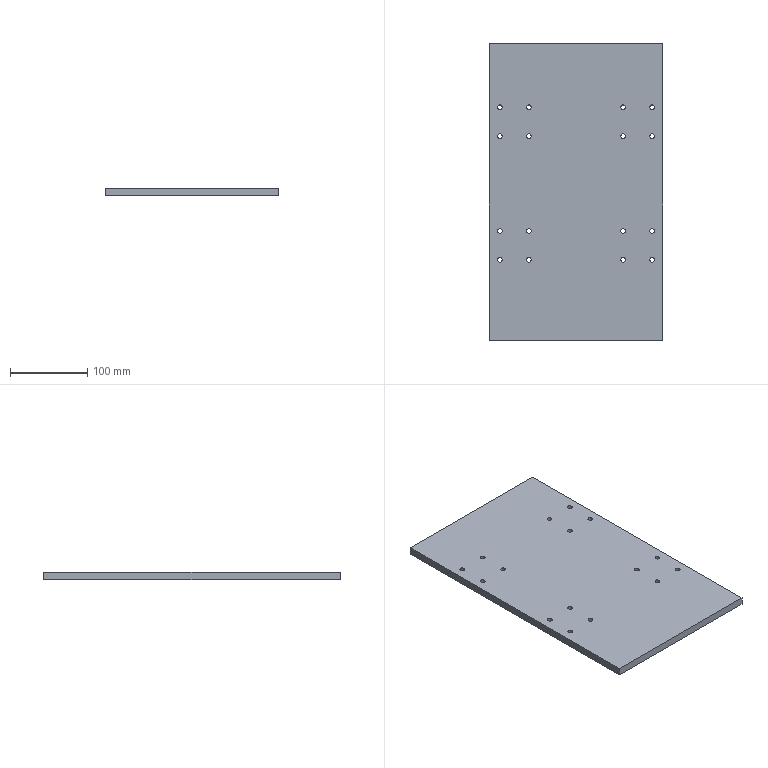Part | STEP file | 1 solid | 38 faces | box 225.075 x 384.491 x 10 mm | volume 860870 mm3 | cylinder 32 | plane 6 | commonest cylinder face diameters 6 x32